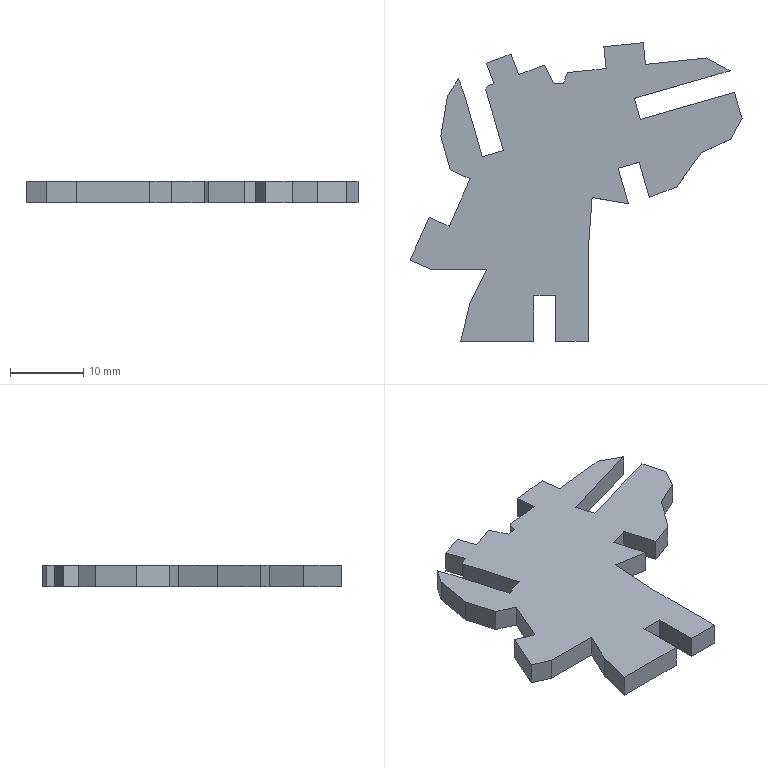Part | SolidWorks | features BaseBody 1 | 1 solid | 51 faces | box 45.454 x 40.899 x 3 mm | volume 2775 mm3 | plane 51